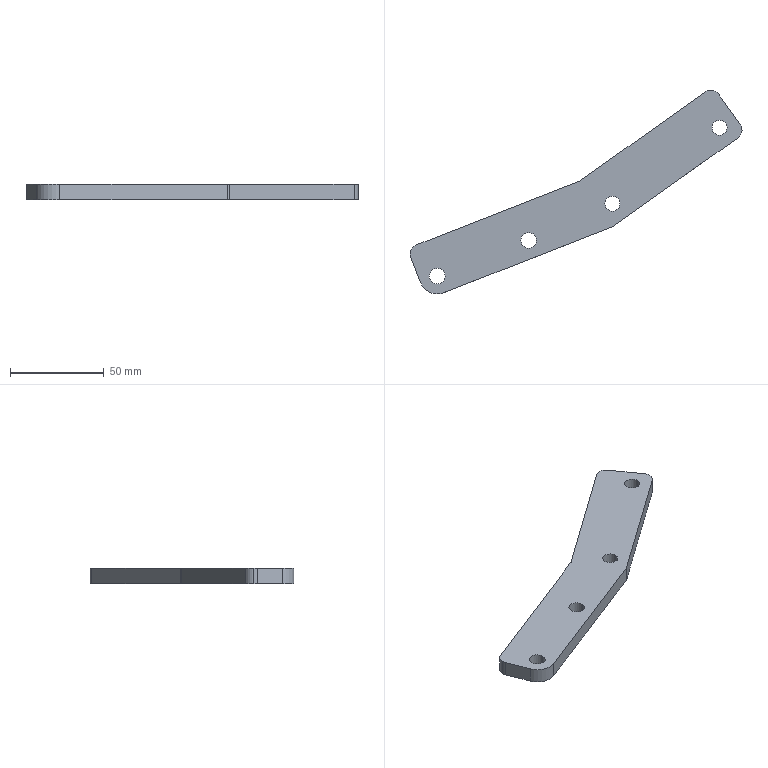Part | SolidWorks | features Cut 1, Extrusion 1 | 1 solid | 23 faces | box 176.98 x 108.741 x 8 mm | volume 42748 mm3 | cylinder 15 | plane 8 | commonest cylinder face diameters 10 x6 8 x4 8.382 x2 8.4 x2 19.05 x1
STEP:
#1=CARTESIAN_POINT('',(84.423,140.052,0.));
#2=VERTEX_POINT('',#1);
#3=CARTESIAN_POINT('',(92.423,140.052,0.));
#4=VERTEX_POINT('',#3);
#5=CARTESIAN_POINT('',(88.423,140.052,0.));
#6=DIRECTION('',(0.,0.,1.));
#7=DIRECTION('',(1.,0.,0.));
#8=AXIS2_PLACEMENT_3D('',#5,#6,#7);
#9=CIRCLE('',#8,4.);
#10=EDGE_CURVE('',#2,#4,#9,.T.);
#11=ORIENTED_EDGE('',*,*,#10,.F.);
#12=CARTESIAN_POINT('',(84.423,140.052,8.));
#13=VERTEX_POINT('',#12);
#14=CARTESIAN_POINT('',(84.423,140.052,-12.));
#15=DIRECTION('',(0.,0.,1.));
#16=VECTOR('',#15,1000.);
#17=LINE('',#14,#16);
#18=EDGE_CURVE('',#2,#13,#17,.T.);
#19=ORIENTED_EDGE('',*,*,#18,.T.);
#20=CARTESIAN_POINT('',(92.423,140.052,8.));
#21=VERTEX_POINT('',#20);
#22=CARTESIAN_POINT('',(88.423,140.052,8.));
#23=DIRECTION('',(0.,0.,1.));
#24=DIRECTION('',(1.,0.,0.));
#25=AXIS2_PLACEMENT_3D('',#22,#23,#24);
#26=CIRCLE('',#25,4.);
#27=EDGE_CURVE('',#13,#21,#26,.T.);
#28=ORIENTED_EDGE('',*,*,#27,.T.);
#29=CARTESIAN_POINT('',(92.423,140.052,-12.));
#30=DIRECTION('',(0.,0.,1.));
#31=VECTOR('',#30,1000.);
#32=LINE('',#29,#31);
#33=EDGE_CURVE('',#4,#21,#32,.T.);
#34=ORIENTED_EDGE('',*,*,#33,.F.);
#35=EDGE_LOOP('',(#11,#19,#28,#34));
#36=FACE_OUTER_BOUND('',#35,.T.);
#37=CARTESIAN_POINT('',(88.423,140.052,-12.));
#38=DIRECTION('',(0.,0.,1.));
#39=DIRECTION('',(1.,0.,0.));
#40=AXIS2_PLACEMENT_3D('',#37,#38,#39);
#41=CYLINDRICAL_SURFACE('',#40,4.);
#42=ADVANCED_FACE('',(#36),#41,.F.);
#43=CARTESIAN_POINT('',(141.505,180.569,0.));
#44=VERTEX_POINT('',#43);
#45=CARTESIAN_POINT('',(149.505,180.569,0.));
#46=VERTEX_POINT('',#45);
#47=CARTESIAN_POINT('',(145.505,180.569,0.));
#48=DIRECTION('',(0.,0.,1.));
#49=DIRECTION('',(1.,0.,0.));
#50=AXIS2_PLACEMENT_3D('',#47,#48,#49);
#51=CIRCLE('',#50,4.);
#52=EDGE_CURVE('',#44,#46,#51,.T.);
#53=ORIENTED_EDGE('',*,*,#52,.F.);
#54=CARTESIAN_POINT('',(141.505,180.569,8.));
#55=VERTEX_POINT('',#54);
#56=CARTESIAN_POINT('',(141.505,180.569,-12.));
#57=DIRECTION('',(0.,0.,1.));
#58=VECTOR('',#57,1000.);
#59=LINE('',#56,#58);
#60=EDGE_CURVE('',#44,#55,#59,.T.);
#61=ORIENTED_EDGE('',*,*,#60,.T.);
#62=CARTESIAN_POINT('',(149.505,180.569,8.));
#63=VERTEX_POINT('',#62);
#64=CARTESIAN_POINT('',(145.505,180.569,8.));
#65=DIRECTION('',(0.,0.,1.));
#66=DIRECTION('',(1.,0.,0.));
#67=AXIS2_PLACEMENT_3D('',#64,#65,#66);
#68=CIRCLE('',#67,4.);
#69=EDGE_CURVE('',#55,#63,#68,.T.);
#70=ORIENTED_EDGE('',*,*,#69,.T.);
#71=CARTESIAN_POINT('',(149.505,180.569,-12.));
#72=DIRECTION('',(0.,0.,1.));
#73=VECTOR('',#72,1000.);
#74=LINE('',#71,#73);
#75=EDGE_CURVE('',#46,#63,#74,.T.);
#76=ORIENTED_EDGE('',*,*,#75,.F.);
#77=EDGE_LOOP('',(#53,#61,#70,#76));
#78=FACE_OUTER_BOUND('',#77,.T.);
#79=CARTESIAN_POINT('',(145.505,180.569,-12.));
#80=DIRECTION('',(0.,0.,1.));
#81=DIRECTION('',(1.,0.,0.));
#82=AXIS2_PLACEMENT_3D('',#79,#80,#81);
#83=CYLINDRICAL_SURFACE('',#82,4.);
#84=ADVANCED_FACE('',(#78),#83,.F.);
#85=CARTESIAN_POINT('',(39.577,120.548,8.));
#86=VERTEX_POINT('',#85);
#87=CARTESIAN_POINT('',(47.959,120.548,8.));
#88=VERTEX_POINT('',#87);
#89=CARTESIAN_POINT('',(43.768,120.548,8.));
#90=DIRECTION('',(0.,0.,1.));
#91=DIRECTION('',(1.,0.,0.));
#92=AXIS2_PLACEMENT_3D('',#89,#90,#91);
#93=CIRCLE('',#92,4.191);
#94=EDGE_CURVE('',#86,#88,#93,.T.);
#95=ORIENTED_EDGE('',*,*,#94,.T.);
#96=CARTESIAN_POINT('',(47.959,120.548,0.));
#97=VERTEX_POINT('',#96);
#98=CARTESIAN_POINT('',(47.959,120.548,8.));
#99=DIRECTION('',(0.,0.,-1.));
#100=VECTOR('',#99,1000.);
#101=LINE('',#98,#100);
#102=EDGE_CURVE('',#88,#97,#101,.T.);
#103=ORIENTED_EDGE('',*,*,#102,.T.);
#104=CARTESIAN_POINT('',(39.577,120.548,0.));
#105=VERTEX_POINT('',#104);
#106=CARTESIAN_POINT('',(43.768,120.548,0.));
#107=DIRECTION('',(0.,0.,1.));
#108=DIRECTION('',(1.,0.,0.));
#109=AXIS2_PLACEMENT_3D('',#106,#107,#108);
#110=CIRCLE('',#109,4.191);
#111=EDGE_CURVE('',#105,#97,#110,.T.);
#112=ORIENTED_EDGE('',*,*,#111,.F.);
#113=CARTESIAN_POINT('',(39.577,120.548,8.));
#114=DIRECTION('',(0.,0.,-1.));
#115=VECTOR('',#114,1000.);
#116=LINE('',#113,#115);
#117=EDGE_CURVE('',#86,#105,#116,.T.);
#118=ORIENTED_EDGE('',*,*,#117,.F.);
#119=EDGE_LOOP('',(#95,#103,#112,#118));
#120=FACE_OUTER_BOUND('',#119,.T.);
#121=CARTESIAN_POINT('',(43.768,120.548,8.));
#122=DIRECTION('',(0.,0.,-1.));
#123=DIRECTION('',(-1.,0.,0.));
#124=AXIS2_PLACEMENT_3D('',#121,#122,#123);
#125=CYLINDRICAL_SURFACE('',#124,4.191);
#126=ADVANCED_FACE('',(#120),#125,.F.);
#127=CARTESIAN_POINT('',(-9.199,101.477,8.));
#128=VERTEX_POINT('',#127);
#129=CARTESIAN_POINT('',(-0.7986,101.477,8.));
#130=VERTEX_POINT('',#129);
#131=CARTESIAN_POINT('',(-4.999,101.477,8.));
#132=DIRECTION('',(0.,0.,1.));
#133=DIRECTION('',(1.,0.,0.));
#134=AXIS2_PLACEMENT_3D('',#131,#132,#133);
#135=CIRCLE('',#134,4.2);
#136=EDGE_CURVE('',#128,#130,#135,.T.);
#137=ORIENTED_EDGE('',*,*,#136,.T.);
#138=CARTESIAN_POINT('',(-0.7986,101.477,0.));
#139=VERTEX_POINT('',#138);
#140=CARTESIAN_POINT('',(-0.7986,101.477,8.));
#141=DIRECTION('',(0.,0.,-1.));
#142=VECTOR('',#141,1000.);
#143=LINE('',#140,#142);
#144=EDGE_CURVE('',#130,#139,#143,.T.);
#145=ORIENTED_EDGE('',*,*,#144,.T.);
#146=CARTESIAN_POINT('',(-9.199,101.477,0.));
#147=VERTEX_POINT('',#146);
#148=CARTESIAN_POINT('',(-4.999,101.477,0.));
#149=DIRECTION('',(0.,0.,1.));
#150=DIRECTION('',(1.,0.,0.));
#151=AXIS2_PLACEMENT_3D('',#148,#149,#150);
#152=CIRCLE('',#151,4.2);
#153=EDGE_CURVE('',#147,#139,#152,.T.);
#154=ORIENTED_EDGE('',*,*,#153,.F.);
#155=CARTESIAN_POINT('',(-9.199,101.477,8.));
#156=DIRECTION('',(0.,0.,-1.));
#157=VECTOR('',#156,1000.);
#158=LINE('',#155,#157);
#159=EDGE_CURVE('',#128,#147,#158,.T.);
#160=ORIENTED_EDGE('',*,*,#159,.F.);
#161=EDGE_LOOP('',(#137,#145,#154,#160));
#162=FACE_OUTER_BOUND('',#161,.T.);
#163=CARTESIAN_POINT('',(-4.999,101.477,8.));
#164=DIRECTION('',(0.,0.,-1.));
#165=DIRECTION('',(-1.,0.,0.));
#166=AXIS2_PLACEMENT_3D('',#163,#164,#165);
#167=CYLINDRICAL_SURFACE('',#166,4.2);
#168=ADVANCED_FACE('',(#162),#167,.F.);
#169=CARTESIAN_POINT('',(-19.503,113.356,8.));
#170=VERTEX_POINT('',#169);
#171=CARTESIAN_POINT('',(-19.16,111.535,8.));
#172=VERTEX_POINT('',#171);
#173=CARTESIAN_POINT('',(-14.503,113.356,8.));
#174=DIRECTION('',(0.,0.,1.));
#175=DIRECTION('',(1.,0.,0.));
#176=AXIS2_PLACEMENT_3D('',#173,#174,#175);
#177=CIRCLE('',#176,5.);
#178=EDGE_CURVE('',#170,#172,#177,.T.);
#179=ORIENTED_EDGE('',*,*,#178,.F.);
#180=CARTESIAN_POINT('',(-19.503,113.356,0.));
#181=VERTEX_POINT('',#180);
#182=CARTESIAN_POINT('',(-19.503,113.356,8.));
#183=DIRECTION('',(0.,0.,-1.));
#184=VECTOR('',#183,1000.);
#185=LINE('',#182,#184);
#186=EDGE_CURVE('',#170,#181,#185,.T.);
#187=ORIENTED_EDGE('',*,*,#186,.T.);
#188=CARTESIAN_POINT('',(-19.16,111.535,0.));
#189=VERTEX_POINT('',#188);
#190=CARTESIAN_POINT('',(-14.503,113.356,0.));
#191=DIRECTION('',(0.,0.,1.));
#192=DIRECTION('',(1.,0.,0.));
#193=AXIS2_PLACEMENT_3D('',#190,#191,#192);
#194=CIRCLE('',#193,5.);
#195=EDGE_CURVE('',#181,#189,#194,.T.);
#196=ORIENTED_EDGE('',*,*,#195,.T.);
#197=CARTESIAN_POINT('',(-19.16,111.535,8.));
#198=DIRECTION('',(0.,0.,-1.));
#199=VECTOR('',#198,1000.);
#200=LINE('',#197,#199);
#201=EDGE_CURVE('',#172,#189,#200,.T.);
#202=ORIENTED_EDGE('',*,*,#201,.F.);
#203=EDGE_LOOP('',(#179,#187,#196,#202));
#204=FACE_OUTER_BOUND('',#203,.T.);
#205=CARTESIAN_POINT('',(-14.503,113.356,8.));
#206=DIRECTION('',(0.,0.,-1.));
#207=DIRECTION('',(-1.,0.,0.));
#208=AXIS2_PLACEMENT_3D('',#205,#206,#207);
#209=CYLINDRICAL_SURFACE('',#208,5.);
#210=ADVANCED_FACE('',(#204),#209,.T.);
#211=CARTESIAN_POINT('',(137.996,199.769,0.));
#212=VERTEX_POINT('',#211);
#213=CARTESIAN_POINT('',(71.495,152.517,0.));
#214=VERTEX_POINT('',#213);
#215=CARTESIAN_POINT('',(-48.027,67.592,0.));
#216=DIRECTION('',(-0.8152,-0.5792,0.));
#217=VECTOR('',#216,1000.);
#218=LINE('',#215,#217);
#219=EDGE_CURVE('',#212,#214,#218,.T.);
#220=ORIENTED_EDGE('',*,*,#219,.T.);
#221=CARTESIAN_POINT('',(71.495,152.517,8.));
#222=VERTEX_POINT('',#221);
#223=CARTESIAN_POINT('',(71.495,152.517,8.));
#224=DIRECTION('',(0.,0.,-1.));
#225=VECTOR('',#224,1000.);
#226=LINE('',#223,#225);
#227=EDGE_CURVE('',#222,#214,#226,.T.);
#228=ORIENTED_EDGE('',*,*,#227,.F.);
#229=CARTESIAN_POINT('',(137.996,199.769,8.));
#230=VERTEX_POINT('',#229);
#231=CARTESIAN_POINT('',(-48.027,67.592,8.));
#232=DIRECTION('',(-0.8152,-0.5792,0.));
#233=VECTOR('',#232,1000.);
#234=LINE('',#231,#233);
#235=EDGE_CURVE('',#230,#222,#234,.T.);
#236=ORIENTED_EDGE('',*,*,#235,.F.);
#237=CARTESIAN_POINT('',(137.996,199.769,8.));
#238=DIRECTION('',(0.,0.,-1.));
#239=VECTOR('',#238,1000.);
#240=LINE('',#237,#239);
#241=EDGE_CURVE('',#230,#212,#240,.T.);
#242=ORIENTED_EDGE('',*,*,#241,.T.);
#243=EDGE_LOOP('',(#220,#228,#236,#242));
#244=FACE_OUTER_BOUND('',#243,.T.);
#245=CARTESIAN_POINT('',(-48.027,67.592,8.));
#246=DIRECTION('',(0.5792,-0.8152,0.));
#247=DIRECTION('',(0.8152,0.5792,0.));
#248=AXIS2_PLACEMENT_3D('',#245,#246,#247);
#249=PLANE('',#248);
#250=ADVANCED_FACE('',(#244),#249,.F.);
#251=CARTESIAN_POINT('',(70.42,151.936,0.));
#252=VERTEX_POINT('',#251);
#253=CARTESIAN_POINT('',(68.599,156.593,0.));
#254=DIRECTION('',(0.,0.,-1.));
#255=DIRECTION('',(1.,0.,0.));
#256=AXIS2_PLACEMENT_3D('',#253,#254,#255);
#257=CIRCLE('',#256,5.);
#258=EDGE_CURVE('',#214,#252,#257,.T.);
#259=ORIENTED_EDGE('',*,*,#258,.T.);
#260=CARTESIAN_POINT('',(70.42,151.936,8.));
#261=VERTEX_POINT('',#260);
#262=CARTESIAN_POINT('',(70.42,151.936,8.));
#263=DIRECTION('',(0.,0.,-1.));
#264=VECTOR('',#263,1000.);
#265=LINE('',#262,#264);
#266=EDGE_CURVE('',#261,#252,#265,.T.);
#267=ORIENTED_EDGE('',*,*,#266,.F.);
#268=CARTESIAN_POINT('',(68.599,156.593,8.));
#269=DIRECTION('',(0.,0.,-1.));
#270=DIRECTION('',(1.,0.,0.));
#271=AXIS2_PLACEMENT_3D('',#268,#269,#270);
#272=CIRCLE('',#271,5.);
#273=EDGE_CURVE('',#222,#261,#272,.T.);
#274=ORIENTED_EDGE('',*,*,#273,.F.);
#275=ORIENTED_EDGE('',*,*,#227,.T.);
#276=EDGE_LOOP('',(#259,#267,#274,#275));
#277=FACE_OUTER_BOUND('',#276,.T.);
#278=CARTESIAN_POINT('',(68.599,156.593,8.));
#279=DIRECTION('',(0.,0.,-1.));
#280=DIRECTION('',(-1.,0.,0.));
#281=AXIS2_PLACEMENT_3D('',#278,#279,#280);
#282=CYLINDRICAL_SURFACE('',#281,5.);
#283=ADVANCED_FACE('',(#277),#282,.F.);
#284=CARTESIAN_POINT('',(-16.324,118.013,0.));
#285=VERTEX_POINT('',#284);
#286=CARTESIAN_POINT('',(-42.195,107.895,0.));
#287=DIRECTION('',(-0.9313,-0.3642,0.));
#288=VECTOR('',#287,1000.);
#289=LINE('',#286,#288);
#290=EDGE_CURVE('',#252,#285,#289,.T.);
#291=ORIENTED_EDGE('',*,*,#290,.T.);
#292=CARTESIAN_POINT('',(-16.324,118.013,8.));
#293=VERTEX_POINT('',#292);
#294=CARTESIAN_POINT('',(-16.324,118.013,8.));
#295=DIRECTION('',(0.,0.,-1.));
#296=VECTOR('',#295,1000.);
#297=LINE('',#294,#296);
#298=EDGE_CURVE('',#293,#285,#297,.T.);
#299=ORIENTED_EDGE('',*,*,#298,.F.);
#300=CARTESIAN_POINT('',(-42.195,107.895,8.));
#301=DIRECTION('',(-0.9313,-0.3642,0.));
#302=VECTOR('',#301,1000.);
#303=LINE('',#300,#302);
#304=EDGE_CURVE('',#261,#293,#303,.T.);
#305=ORIENTED_EDGE('',*,*,#304,.F.);
#306=ORIENTED_EDGE('',*,*,#266,.T.);
#307=EDGE_LOOP('',(#291,#299,#305,#306));
#308=FACE_OUTER_BOUND('',#307,.T.);
#309=CARTESIAN_POINT('',(-42.195,107.895,8.));
#310=DIRECTION('',(0.3642,-0.9313,0.));
#311=DIRECTION('',(0.9313,0.3642,0.));
#312=AXIS2_PLACEMENT_3D('',#309,#310,#311);
#313=PLANE('',#312);
#314=ADVANCED_FACE('',(#308),#313,.F.);
#315=ORIENTED_EDGE('',*,*,#186,.F.);
#316=CARTESIAN_POINT('',(-14.503,113.356,8.));
#317=DIRECTION('',(0.,0.,1.));
#318=DIRECTION('',(1.,0.,0.));
#319=AXIS2_PLACEMENT_3D('',#316,#317,#318);
#320=CIRCLE('',#319,5.);
#321=EDGE_CURVE('',#293,#170,#320,.T.);
#322=ORIENTED_EDGE('',*,*,#321,.F.);
#323=ORIENTED_EDGE('',*,*,#298,.T.);
#324=CARTESIAN_POINT('',(-14.503,113.356,0.));
#325=DIRECTION('',(0.,0.,1.));
#326=DIRECTION('',(1.,0.,0.));
#327=AXIS2_PLACEMENT_3D('',#324,#325,#326);
#328=CIRCLE('',#327,5.);
#329=EDGE_CURVE('',#285,#181,#328,.T.);
#330=ORIENTED_EDGE('',*,*,#329,.T.);
#331=EDGE_LOOP('',(#315,#322,#323,#330));
#332=FACE_OUTER_BOUND('',#331,.T.);
#333=CARTESIAN_POINT('',(-14.503,113.356,8.));
#334=DIRECTION('',(0.,0.,-1.));
#335=DIRECTION('',(-1.,0.,0.));
#336=AXIS2_PLACEMENT_3D('',#333,#334,#335);
#337=CYLINDRICAL_SURFACE('',#336,5.);
#338=ADVANCED_FACE('',(#332),#337,.T.);
#339=CARTESIAN_POINT('',(-13.869,98.008,0.));
#340=VERTEX_POINT('',#339);
#341=CARTESIAN_POINT('',(21.214,8.296,0.));
#342=DIRECTION('',(-0.3642,0.9313,0.));
#343=VECTOR('',#342,1000.);
#344=LINE('',#341,#343);
#345=EDGE_CURVE('',#340,#189,#344,.T.);
#346=ORIENTED_EDGE('',*,*,#345,.F.);
#347=CARTESIAN_POINT('',(-13.869,98.008,8.));
#348=VERTEX_POINT('',#347);
#349=CARTESIAN_POINT('',(-13.869,98.008,8.));
#350=DIRECTION('',(0.,0.,-1.));
#351=VECTOR('',#350,1000.);
#352=LINE('',#349,#351);
#353=EDGE_CURVE('',#348,#340,#352,.T.);
#354=ORIENTED_EDGE('',*,*,#353,.F.);
#355=CARTESIAN_POINT('',(21.214,8.296,8.));
#356=DIRECTION('',(-0.3642,0.9313,0.));
#357=VECTOR('',#356,1000.);
#358=LINE('',#355,#357);
#359=EDGE_CURVE('',#348,#172,#358,.T.);
#360=ORIENTED_EDGE('',*,*,#359,.T.);
#361=ORIENTED_EDGE('',*,*,#201,.T.);
#362=EDGE_LOOP('',(#346,#354,#360,#361));
#363=FACE_OUTER_BOUND('',#362,.T.);
#364=CARTESIAN_POINT('',(21.214,8.296,8.));
#365=DIRECTION('',(-0.9313,-0.3642,0.));
#366=DIRECTION('',(0.3642,-0.9313,0.));
#367=AXIS2_PLACEMENT_3D('',#364,#365,#366);
#368=PLANE('',#367);
#369=ADVANCED_FACE('',(#363),#368,.T.);
#370=CARTESIAN_POINT('',(-1.529,92.606,0.));
#371=VERTEX_POINT('',#370);
#372=CARTESIAN_POINT('',(-4.999,101.477,0.));
#373=DIRECTION('',(0.,0.,1.));
#374=DIRECTION('',(1.,0.,0.));
#375=AXIS2_PLACEMENT_3D('',#372,#373,#374);
#376=CIRCLE('',#375,9.525);
#377=EDGE_CURVE('',#340,#371,#376,.T.);
#378=ORIENTED_EDGE('',*,*,#377,.T.);
#379=CARTESIAN_POINT('',(-1.529,92.606,8.));
#380=VERTEX_POINT('',#379);
#381=CARTESIAN_POINT('',(-1.529,92.606,8.));
#382=DIRECTION('',(0.,0.,-1.));
#383=VECTOR('',#382,1000.);
#384=LINE('',#381,#383);
#385=EDGE_CURVE('',#380,#371,#384,.T.);
#386=ORIENTED_EDGE('',*,*,#385,.F.);
#387=CARTESIAN_POINT('',(-4.999,101.477,8.));
#388=DIRECTION('',(0.,0.,1.));
#389=DIRECTION('',(1.,0.,0.));
#390=AXIS2_PLACEMENT_3D('',#387,#388,#389);
#391=CIRCLE('',#390,9.525);
#392=EDGE_CURVE('',#348,#380,#391,.T.);
#393=ORIENTED_EDGE('',*,*,#392,.F.);
#394=ORIENTED_EDGE('',*,*,#353,.T.);
#395=EDGE_LOOP('',(#378,#386,#393,#394));
#396=FACE_OUTER_BOUND('',#395,.T.);
#397=CARTESIAN_POINT('',(-4.999,101.477,8.));
#398=DIRECTION('',(0.,0.,-1.));
#399=DIRECTION('',(-1.,0.,0.));
#400=AXIS2_PLACEMENT_3D('',#397,#398,#399);
#401=CYLINDRICAL_SURFACE('',#400,9.525);
#402=ADVANCED_FACE('',(#396),#401,.T.);
#403=CARTESIAN_POINT('',(87.979,127.611,0.));
#404=VERTEX_POINT('',#403);
#405=CARTESIAN_POINT('',(-31.615,80.841,0.));
#406=DIRECTION('',(-0.9313,-0.3642,0.));
#407=VECTOR('',#406,1000.);
#408=LINE('',#405,#407);
#409=EDGE_CURVE('',#404,#371,#408,.T.);
#410=ORIENTED_EDGE('',*,*,#409,.F.);
#411=CARTESIAN_POINT('',(87.979,127.611,8.));
#412=VERTEX_POINT('',#411);
#413=CARTESIAN_POINT('',(87.979,127.611,8.));
#414=DIRECTION('',(0.,0.,-1.));
#415=VECTOR('',#414,1000.);
#416=LINE('',#413,#415);
#417=EDGE_CURVE('',#412,#404,#416,.T.);
#418=ORIENTED_EDGE('',*,*,#417,.F.);
#419=CARTESIAN_POINT('',(-31.615,80.841,8.));
#420=DIRECTION('',(-0.9313,-0.3642,0.));
#421=VECTOR('',#420,1000.);
#422=LINE('',#419,#421);
#423=EDGE_CURVE('',#412,#380,#422,.T.);
#424=ORIENTED_EDGE('',*,*,#423,.T.);
#425=ORIENTED_EDGE('',*,*,#385,.T.);
#426=EDGE_LOOP('',(#410,#418,#424,#425));
#427=FACE_OUTER_BOUND('',#426,.T.);
#428=CARTESIAN_POINT('',(-31.615,80.841,8.));
#429=DIRECTION('',(0.3642,-0.9313,0.));
#430=DIRECTION('',(0.9313,0.3642,0.));
#431=AXIS2_PLACEMENT_3D('',#428,#429,#430);
#432=PLANE('',#431);
#433=ADVANCED_FACE('',(#427),#432,.T.);
#434=CARTESIAN_POINT('',(89.054,128.191,0.));
#435=VERTEX_POINT('',#434);
#436=CARTESIAN_POINT('',(86.158,132.267,0.));
#437=DIRECTION('',(0.,0.,1.));
#438=DIRECTION('',(1.,0.,0.));
#439=AXIS2_PLACEMENT_3D('',#436,#437,#438);
#440=CIRCLE('',#439,5.);
#441=EDGE_CURVE('',#404,#435,#440,.T.);
#442=ORIENTED_EDGE('',*,*,#441,.T.);
#443=CARTESIAN_POINT('',(89.054,128.191,8.));
#444=VERTEX_POINT('',#443);
#445=CARTESIAN_POINT('',(89.054,128.191,8.));
#446=DIRECTION('',(0.,0.,-1.));
#447=VECTOR('',#446,1000.);
#448=LINE('',#445,#447);
#449=EDGE_CURVE('',#444,#435,#448,.T.);
#450=ORIENTED_EDGE('',*,*,#449,.F.);
#451=CARTESIAN_POINT('',(86.158,132.267,8.));
#452=DIRECTION('',(0.,0.,1.));
#453=DIRECTION('',(1.,0.,0.));
#454=AXIS2_PLACEMENT_3D('',#451,#452,#453);
#455=CIRCLE('',#454,5.);
#456=EDGE_CURVE('',#412,#444,#455,.T.);
#457=ORIENTED_EDGE('',*,*,#456,.F.);
#458=ORIENTED_EDGE('',*,*,#417,.T.);
#459=EDGE_LOOP('',(#442,#450,#457,#458));
#460=FACE_OUTER_BOUND('',#459,.T.);
#461=CARTESIAN_POINT('',(86.158,132.267,8.));
#462=DIRECTION('',(0.,0.,-1.));
#463=DIRECTION('',(-1.,0.,0.));
#464=AXIS2_PLACEMENT_3D('',#461,#462,#463);
#465=CYLINDRICAL_SURFACE('',#464,5.);
#466=ADVANCED_FACE('',(#460),#465,.T.);
#467=CARTESIAN_POINT('',(155.373,175.313,0.));
#468=VERTEX_POINT('',#467);
#469=CARTESIAN_POINT('',(-30.65,43.136,0.));
#470=DIRECTION('',(-0.8152,-0.5792,0.));
#471=VECTOR('',#470,1000.);
#472=LINE('',#469,#471);
#473=EDGE_CURVE('',#468,#435,#472,.T.);
#474=ORIENTED_EDGE('',*,*,#473,.F.);
#475=CARTESIAN_POINT('',(155.373,175.313,8.));
#476=VERTEX_POINT('',#475);
#477=CARTESIAN_POINT('',(155.373,175.313,8.));
#478=DIRECTION('',(0.,0.,-1.));
#479=VECTOR('',#478,1000.);
#480=LINE('',#477,#479);
#481=EDGE_CURVE('',#476,#468,#480,.T.);
#482=ORIENTED_EDGE('',*,*,#481,.F.);
#483=CARTESIAN_POINT('',(-30.65,43.136,8.));
#484=DIRECTION('',(-0.8152,-0.5792,0.));
#485=VECTOR('',#484,1000.);
#486=LINE('',#483,#485);
#487=EDGE_CURVE('',#476,#444,#486,.T.);
#488=ORIENTED_EDGE('',*,*,#487,.T.);
#489=ORIENTED_EDGE('',*,*,#449,.T.);
#490=EDGE_LOOP('',(#474,#482,#488,#489));
#491=FACE_OUTER_BOUND('',#490,.T.);
#492=CARTESIAN_POINT('',(-30.65,43.136,8.));
#493=DIRECTION('',(0.5792,-0.8152,0.));
#494=DIRECTION('',(0.8152,0.5792,0.));
#495=AXIS2_PLACEMENT_3D('',#492,#493,#494);
#496=PLANE('',#495);
#497=ADVANCED_FACE('',(#491),#496,.T.);
#498=CARTESIAN_POINT('',(156.552,182.285,0.));
#499=VERTEX_POINT('',#498);
#500=CARTESIAN_POINT('',(152.477,179.389,0.));
#501=DIRECTION('',(0.,0.,-1.));
#502=DIRECTION('',(1.,0.,0.));
#503=AXIS2_PLACEMENT_3D('',#500,#501,#502);
#504=CIRCLE('',#503,5.);
#505=EDGE_CURVE('',#499,#468,#504,.T.);
#506=ORIENTED_EDGE('',*,*,#505,.F.);
#507=CARTESIAN_POINT('',(156.552,182.285,8.));
#508=VERTEX_POINT('',#507);
#509=CARTESIAN_POINT('',(156.552,182.285,8.));
#510=DIRECTION('',(0.,0.,-1.));
#511=VECTOR('',#510,1000.);
#512=LINE('',#509,#511);
#513=EDGE_CURVE('',#508,#499,#512,.T.);
#514=ORIENTED_EDGE('',*,*,#513,.F.);
#515=CARTESIAN_POINT('',(152.477,179.389,8.));
#516=DIRECTION('',(0.,0.,-1.));
#517=DIRECTION('',(1.,0.,0.));
#518=AXIS2_PLACEMENT_3D('',#515,#516,#517);
#519=CIRCLE('',#518,5.);
#520=EDGE_CURVE('',#508,#476,#519,.T.);
#521=ORIENTED_EDGE('',*,*,#520,.T.);
#522=ORIENTED_EDGE('',*,*,#481,.T.);
#523=EDGE_LOOP('',(#506,#514,#521,#522));
#524=FACE_OUTER_BOUND('',#523,.T.);
#525=CARTESIAN_POINT('',(152.477,179.389,8.));
#526=DIRECTION('',(0.,0.,-1.));
#527=DIRECTION('',(-1.,0.,0.));
#528=AXIS2_PLACEMENT_3D('',#525,#526,#527);
#529=CYLINDRICAL_SURFACE('',#528,5.);
#530=ADVANCED_FACE('',(#524),#529,.T.);
#531=CARTESIAN_POINT('',(144.968,198.589,0.));
#532=VERTEX_POINT('',#531);
#533=CARTESIAN_POINT('',(190.099,135.073,0.));
#534=DIRECTION('',(-0.5792,0.8152,0.));
#535=VECTOR('',#534,1000.);
#536=LINE('',#533,#535);
#537=EDGE_CURVE('',#499,#532,#536,.T.);
#538=ORIENTED_EDGE('',*,*,#537,.T.);
#539=CARTESIAN_POINT('',(144.968,198.589,8.));
#540=VERTEX_POINT('',#539);
#541=CARTESIAN_POINT('',(144.968,198.589,8.));
#542=DIRECTION('',(0.,0.,-1.));
#543=VECTOR('',#542,1000.);
#544=LINE('',#541,#543);
#545=EDGE_CURVE('',#540,#532,#544,.T.);
#546=ORIENTED_EDGE('',*,*,#545,.F.);
#547=CARTESIAN_POINT('',(190.099,135.073,8.));
#548=DIRECTION('',(-0.5792,0.8152,0.));
#549=VECTOR('',#548,1000.);
#550=LINE('',#547,#549);
#551=EDGE_CURVE('',#508,#540,#550,.T.);
#552=ORIENTED_EDGE('',*,*,#551,.F.);
#553=ORIENTED_EDGE('',*,*,#513,.T.);
#554=EDGE_LOOP('',(#538,#546,#552,#553));
#555=FACE_OUTER_BOUND('',#554,.T.);
#556=CARTESIAN_POINT('',(190.099,135.073,8.));
#557=DIRECTION('',(-0.8152,-0.5792,0.));
#558=DIRECTION('',(0.5792,-0.8152,0.));
#559=AXIS2_PLACEMENT_3D('',#556,#557,#558);
#560=PLANE('',#559);
#561=ADVANCED_FACE('',(#555),#560,.F.);
#562=ORIENTED_EDGE('',*,*,#144,.F.);
#563=CARTESIAN_POINT('',(-4.999,101.477,8.));
#564=DIRECTION('',(0.,0.,1.));
#565=DIRECTION('',(1.,0.,0.));
#566=AXIS2_PLACEMENT_3D('',#563,#564,#565);
#567=CIRCLE('',#566,4.2);
#568=EDGE_CURVE('',#130,#128,#567,.T.);
#569=ORIENTED_EDGE('',*,*,#568,.T.);
#570=ORIENTED_EDGE('',*,*,#159,.T.);
#571=CARTESIAN_POINT('',(-4.999,101.477,0.));
#572=DIRECTION('',(0.,0.,1.));
#573=DIRECTION('',(1.,0.,0.));
#574=AXIS2_PLACEMENT_3D('',#571,#572,#573);
#575=CIRCLE('',#574,4.2);
#576=EDGE_CURVE('',#139,#147,#575,.T.);
#577=ORIENTED_EDGE('',*,*,#576,.F.);
#578=EDGE_LOOP('',(#562,#569,#570,#577));
#579=FACE_OUTER_BOUND('',#578,.T.);
#580=CARTESIAN_POINT('',(-4.999,101.477,8.));
#581=DIRECTION('',(0.,0.,-1.));
#582=DIRECTION('',(-1.,0.,0.));
#583=AXIS2_PLACEMENT_3D('',#580,#581,#582);
#584=CYLINDRICAL_SURFACE('',#583,4.2);
#585=ADVANCED_FACE('',(#579),#584,.F.);
#586=ORIENTED_EDGE('',*,*,#102,.F.);
#587=CARTESIAN_POINT('',(43.768,120.548,8.));
#588=DIRECTION('',(0.,0.,1.));
#589=DIRECTION('',(1.,0.,0.));
#590=AXIS2_PLACEMENT_3D('',#587,#588,#589);
#591=CIRCLE('',#590,4.191);
#592=EDGE_CURVE('',#88,#86,#591,.T.);
#593=ORIENTED_EDGE('',*,*,#592,.T.);
#594=ORIENTED_EDGE('',*,*,#117,.T.);
#595=CARTESIAN_POINT('',(43.768,120.548,0.));
#596=DIRECTION('',(0.,0.,1.));
#597=DIRECTION('',(1.,0.,0.));
#598=AXIS2_PLACEMENT_3D('',#595,#596,#597);
#599=CIRCLE('',#598,4.191);
#600=EDGE_CURVE('',#97,#105,#599,.T.);
#601=ORIENTED_EDGE('',*,*,#600,.F.);
#602=EDGE_LOOP('',(#586,#593,#594,#601));
#603=FACE_OUTER_BOUND('',#602,.T.);
#604=CARTESIAN_POINT('',(43.768,120.548,8.));
#605=DIRECTION('',(0.,0.,-1.));
#606=DIRECTION('',(-1.,0.,0.));
#607=AXIS2_PLACEMENT_3D('',#604,#605,#606);
#608=CYLINDRICAL_SURFACE('',#607,4.191);
#609=ADVANCED_FACE('',(#603),#608,.F.);
#610=CARTESIAN_POINT('',(140.892,195.693,0.));
#611=DIRECTION('',(0.,0.,1.));
#612=DIRECTION('',(1.,0.,0.));
#613=AXIS2_PLACEMENT_3D('',#610,#611,#612);
#614=CIRCLE('',#613,5.);
#615=EDGE_CURVE('',#532,#212,#614,.T.);
#616=ORIENTED_EDGE('',*,*,#615,.T.);
#617=ORIENTED_EDGE('',*,*,#241,.F.);
#618=CARTESIAN_POINT('',(140.892,195.693,8.));
#619=DIRECTION('',(0.,0.,1.));
#620=DIRECTION('',(1.,0.,0.));
#621=AXIS2_PLACEMENT_3D('',#618,#619,#620);
#622=CIRCLE('',#621,5.);
#623=EDGE_CURVE('',#540,#230,#622,.T.);
#624=ORIENTED_EDGE('',*,*,#623,.F.);
#625=ORIENTED_EDGE('',*,*,#545,.T.);
#626=EDGE_LOOP('',(#616,#617,#624,#625));
#627=FACE_OUTER_BOUND('',#626,.T.);
#628=CARTESIAN_POINT('',(140.892,195.693,8.));
#629=DIRECTION('',(0.,0.,-1.));
#630=DIRECTION('',(-1.,0.,0.));
#631=AXIS2_PLACEMENT_3D('',#628,#629,#630);
#632=CYLINDRICAL_SURFACE('',#631,5.);
#633=ADVANCED_FACE('',(#627),#632,.T.);
#634=CARTESIAN_POINT('',(88.423,140.052,8.));
#635=DIRECTION('',(0.,0.,1.));
#636=DIRECTION('',(1.,0.,0.));
#637=AXIS2_PLACEMENT_3D('',#634,#635,#636);
#638=CIRCLE('',#637,4.);
#639=EDGE_CURVE('',#21,#13,#638,.T.);
#640=ORIENTED_EDGE('',*,*,#639,.F.);
#641=ORIENTED_EDGE('',*,*,#27,.F.);
#642=EDGE_LOOP('',(#640,#641));
#643=FACE_BOUND('',#642,.T.);
#644=CARTESIAN_POINT('',(145.505,180.569,8.));
#645=DIRECTION('',(0.,0.,1.));
#646=DIRECTION('',(1.,0.,0.));
#647=AXIS2_PLACEMENT_3D('',#644,#645,#646);
#648=CIRCLE('',#647,4.);
#649=EDGE_CURVE('',#63,#55,#648,.T.);
#650=ORIENTED_EDGE('',*,*,#649,.F.);
#651=ORIENTED_EDGE('',*,*,#69,.F.);
#652=EDGE_LOOP('',(#650,#651));
#653=FACE_BOUND('',#652,.T.);
#654=ORIENTED_EDGE('',*,*,#94,.F.);
#655=ORIENTED_EDGE('',*,*,#592,.F.);
#656=EDGE_LOOP('',(#654,#655));
#657=FACE_BOUND('',#656,.T.);
#658=ORIENTED_EDGE('',*,*,#136,.F.);
#659=ORIENTED_EDGE('',*,*,#568,.F.);
#660=EDGE_LOOP('',(#658,#659));
#661=FACE_BOUND('',#660,.T.);
#662=ORIENTED_EDGE('',*,*,#235,.T.);
#663=ORIENTED_EDGE('',*,*,#273,.T.);
#664=ORIENTED_EDGE('',*,*,#304,.T.);
#665=ORIENTED_EDGE('',*,*,#321,.T.);
#666=ORIENTED_EDGE('',*,*,#178,.T.);
#667=ORIENTED_EDGE('',*,*,#359,.F.);
#668=ORIENTED_EDGE('',*,*,#392,.T.);
#669=ORIENTED_EDGE('',*,*,#423,.F.);
#670=ORIENTED_EDGE('',*,*,#456,.T.);
#671=ORIENTED_EDGE('',*,*,#487,.F.);
#672=ORIENTED_EDGE('',*,*,#520,.F.);
#673=ORIENTED_EDGE('',*,*,#551,.T.);
#674=ORIENTED_EDGE('',*,*,#623,.T.);
#675=EDGE_LOOP('',(#662,#663,#664,#665,#666,#667,#668,#669,#670,#671,#672,#673,#674));
#676=FACE_OUTER_BOUND('',#675,.T.);
#677=CARTESIAN_POINT('',(0.,0.,8.));
#678=DIRECTION('',(0.,0.,1.));
#679=DIRECTION('',(1.,0.,0.));
#680=AXIS2_PLACEMENT_3D('',#677,#678,#679);
#681=PLANE('',#680);
#682=ADVANCED_FACE('',(#643,#653,#657,#661,#676),#681,.T.);
#683=CARTESIAN_POINT('',(88.423,140.052,0.));
#684=DIRECTION('',(0.,0.,1.));
#685=DIRECTION('',(1.,0.,0.));
#686=AXIS2_PLACEMENT_3D('',#683,#684,#685);
#687=CIRCLE('',#686,4.);
#688=EDGE_CURVE('',#4,#2,#687,.T.);
#689=ORIENTED_EDGE('',*,*,#688,.T.);
#690=ORIENTED_EDGE('',*,*,#10,.T.);
#691=EDGE_LOOP('',(#689,#690));
#692=FACE_BOUND('',#691,.T.);
#693=CARTESIAN_POINT('',(145.505,180.569,0.));
#694=DIRECTION('',(0.,0.,1.));
#695=DIRECTION('',(1.,0.,0.));
#696=AXIS2_PLACEMENT_3D('',#693,#694,#695);
#697=CIRCLE('',#696,4.);
#698=EDGE_CURVE('',#46,#44,#697,.T.);
#699=ORIENTED_EDGE('',*,*,#698,.T.);
#700=ORIENTED_EDGE('',*,*,#52,.T.);
#701=EDGE_LOOP('',(#699,#700));
#702=FACE_BOUND('',#701,.T.);
#703=ORIENTED_EDGE('',*,*,#111,.T.);
#704=ORIENTED_EDGE('',*,*,#600,.T.);
#705=EDGE_LOOP('',(#703,#704));
#706=FACE_BOUND('',#705,.T.);
#707=ORIENTED_EDGE('',*,*,#153,.T.);
#708=ORIENTED_EDGE('',*,*,#576,.T.);
#709=EDGE_LOOP('',(#707,#708));
#710=FACE_BOUND('',#709,.T.);
#711=ORIENTED_EDGE('',*,*,#219,.F.);
#712=ORIENTED_EDGE('',*,*,#615,.F.);
#713=ORIENTED_EDGE('',*,*,#537,.F.);
#714=ORIENTED_EDGE('',*,*,#505,.T.);
#715=ORIENTED_EDGE('',*,*,#473,.T.);
#716=ORIENTED_EDGE('',*,*,#441,.F.);
#717=ORIENTED_EDGE('',*,*,#409,.T.);
#718=ORIENTED_EDGE('',*,*,#377,.F.);
#719=ORIENTED_EDGE('',*,*,#345,.T.);
#720=ORIENTED_EDGE('',*,*,#195,.F.);
#721=ORIENTED_EDGE('',*,*,#329,.F.);
#722=ORIENTED_EDGE('',*,*,#290,.F.);
#723=ORIENTED_EDGE('',*,*,#258,.F.);
#724=EDGE_LOOP('',(#711,#712,#713,#714,#715,#716,#717,#718,#719,#720,#721,#722,#723));
#725=FACE_OUTER_BOUND('',#724,.T.);
#726=CARTESIAN_POINT('',(0.,0.,0.));
#727=DIRECTION('',(0.,0.,1.));
#728=DIRECTION('',(1.,0.,0.));
#729=AXIS2_PLACEMENT_3D('',#726,#727,#728);
#730=PLANE('',#729);
#731=ADVANCED_FACE('',(#692,#702,#706,#710,#725),#730,.F.);
#732=ORIENTED_EDGE('',*,*,#60,.F.);
#733=ORIENTED_EDGE('',*,*,#698,.F.);
#734=ORIENTED_EDGE('',*,*,#75,.T.);
#735=ORIENTED_EDGE('',*,*,#649,.T.);
#736=EDGE_LOOP('',(#732,#733,#734,#735));
#737=FACE_OUTER_BOUND('',#736,.T.);
#738=CARTESIAN_POINT('',(145.505,180.569,-12.));
#739=DIRECTION('',(0.,0.,1.));
#740=DIRECTION('',(1.,0.,0.));
#741=AXIS2_PLACEMENT_3D('',#738,#739,#740);
#742=CYLINDRICAL_SURFACE('',#741,4.);
#743=ADVANCED_FACE('',(#737),#742,.F.);
#744=ORIENTED_EDGE('',*,*,#18,.F.);
#745=ORIENTED_EDGE('',*,*,#688,.F.);
#746=ORIENTED_EDGE('',*,*,#33,.T.);
#747=ORIENTED_EDGE('',*,*,#639,.T.);
#748=EDGE_LOOP('',(#744,#745,#746,#747));
#749=FACE_OUTER_BOUND('',#748,.T.);
#750=CARTESIAN_POINT('',(88.423,140.052,-12.));
#751=DIRECTION('',(0.,0.,1.));
#752=DIRECTION('',(1.,0.,0.));
#753=AXIS2_PLACEMENT_3D('',#750,#751,#752);
#754=CYLINDRICAL_SURFACE('',#753,4.);
#755=ADVANCED_FACE('',(#749),#754,.F.);
#756=CLOSED_SHELL('',(#42,#84,#126,#168,#210,#250,#283,#314,#338,#369,#402,#433,#466,#497,#530,#561,#585,#609,#633,#682,#731,#743,#755));
#757=MANIFOLD_SOLID_BREP('',#756);
#758=CARTESIAN_POINT('',(0.,0.,0.));
#759=DIRECTION('',(0.,0.,1.));
#760=DIRECTION('',(1.,0.,0.));
#761=AXIS2_PLACEMENT_3D('',#758,#759,#760);
#762=(LENGTH_UNIT()NAMED_UNIT(*)SI_UNIT(.MILLI.,.METRE.));
#763=UNCERTAINTY_MEASURE_WITH_UNIT(LENGTH_MEASURE(0.00001),#762,'','');
#764=(NAMED_UNIT(*)PLANE_ANGLE_UNIT()SI_UNIT($,.RADIAN.));
#765=(NAMED_UNIT(*)SI_UNIT($,.STERADIAN.)SOLID_ANGLE_UNIT());
#766=(GEOMETRIC_REPRESENTATION_CONTEXT(3)GLOBAL_UNCERTAINTY_ASSIGNED_CONTEXT((#763))GLOBAL_UNIT_ASSIGNED_CONTEXT((#762,#764,#765))REPRESENTATION_CONTEXT('',''));
#767=ADVANCED_BREP_SHAPE_REPRESENTATION('',(#757,#761),#766);